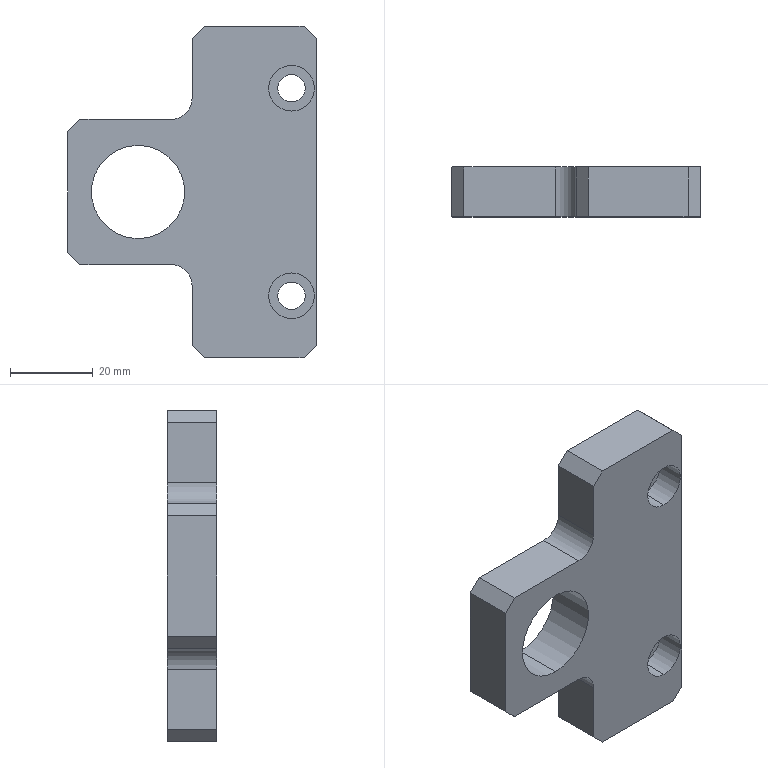Part | STEP file | PN_0049 | 1 solid | 30 faces | box 60 x 12 x 80 mm | volume 34785 mm3 | plane 18 | cylinder 12 | commonest cylinder face diameters 6.6 x4 11 x4 10 x2 22.5 x2